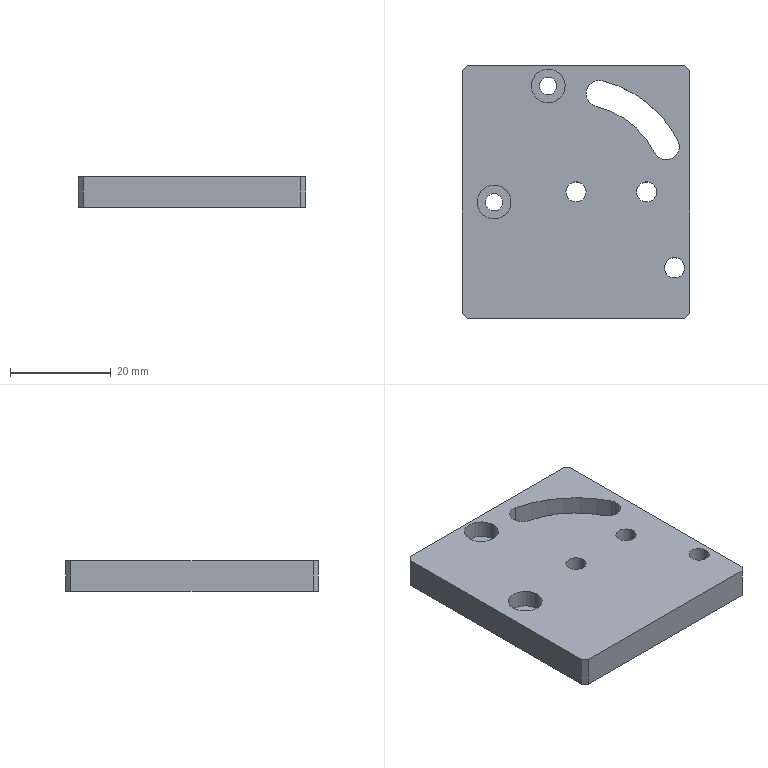Part | NX | features BREP 1 | 1 solid | 31 faces | box 45 x 50 x 6 mm | volume 12298 mm3 | cylinder 19 | plane 12 | commonest cylinder face diameters 4 x6 3.4 x4 6.7 x4 5.2 x3 34.8 x1 45.2 x1
STEP:
#1=CARTESIAN_POINT('',(-8.85,21.,2.5));
#2=VERTEX_POINT('',#1);
#3=CARTESIAN_POINT('',(-2.15,21.,2.5));
#4=VERTEX_POINT('',#3);
#5=CARTESIAN_POINT('',(-5.5,21.,2.5));
#6=DIRECTION('',(0.,0.,1.));
#7=DIRECTION('',(1.,0.,0.));
#8=AXIS2_PLACEMENT_3D('',#5,#6,#7);
#9=CIRCLE('',#8,3.35);
#10=EDGE_CURVE('',#2,#4,#9,.T.);
#11=ORIENTED_EDGE('',*,*,#10,.F.);
#12=CARTESIAN_POINT('',(-8.85,21.,6.));
#13=VERTEX_POINT('',#12);
#14=CARTESIAN_POINT('',(-8.85,21.,6.));
#15=DIRECTION('',(0.,0.,1.));
#16=VECTOR('',#15,1000.);
#17=LINE('',#14,#16);
#18=EDGE_CURVE('',#13,#2,#17,.F.);
#19=ORIENTED_EDGE('',*,*,#18,.F.);
#20=CARTESIAN_POINT('',(-2.15,21.,6.));
#21=VERTEX_POINT('',#20);
#22=CARTESIAN_POINT('',(-5.5,21.,6.));
#23=DIRECTION('',(0.,0.,1.));
#24=DIRECTION('',(1.,0.,0.));
#25=AXIS2_PLACEMENT_3D('',#22,#23,#24);
#26=CIRCLE('',#25,3.35);
#27=EDGE_CURVE('',#13,#21,#26,.T.);
#28=ORIENTED_EDGE('',*,*,#27,.T.);
#29=CARTESIAN_POINT('',(-2.15,21.,6.));
#30=DIRECTION('',(0.,0.,1.));
#31=VECTOR('',#30,1000.);
#32=LINE('',#29,#31);
#33=EDGE_CURVE('',#21,#4,#32,.F.);
#34=ORIENTED_EDGE('',*,*,#33,.T.);
#35=EDGE_LOOP('',(#11,#19,#28,#34));
#36=FACE_BOUND('',#35,.T.);
#37=CARTESIAN_POINT('',(-5.5,21.,6.));
#38=DIRECTION('',(0.,0.,1.));
#39=DIRECTION('',(1.,0.,0.));
#40=AXIS2_PLACEMENT_3D('',#37,#38,#39);
#41=CYLINDRICAL_SURFACE('',#40,3.35);
#42=ADVANCED_FACE('',(#36),#41,.F.);
#43=CARTESIAN_POINT('',(-7.2,21.,0.));
#44=VERTEX_POINT('',#43);
#45=CARTESIAN_POINT('',(-3.8,21.,0.));
#46=VERTEX_POINT('',#45);
#47=CARTESIAN_POINT('',(-5.5,21.,0.));
#48=DIRECTION('',(0.,0.,1.));
#49=DIRECTION('',(1.,0.,0.));
#50=AXIS2_PLACEMENT_3D('',#47,#48,#49);
#51=CIRCLE('',#50,1.7);
#52=EDGE_CURVE('',#44,#46,#51,.T.);
#53=ORIENTED_EDGE('',*,*,#52,.F.);
#54=CARTESIAN_POINT('',(-7.2,21.,2.5));
#55=VERTEX_POINT('',#54);
#56=CARTESIAN_POINT('',(-7.2,21.,6.));
#57=DIRECTION('',(0.,0.,1.));
#58=VECTOR('',#57,1000.);
#59=LINE('',#56,#58);
#60=EDGE_CURVE('',#55,#44,#59,.F.);
#61=ORIENTED_EDGE('',*,*,#60,.F.);
#62=CARTESIAN_POINT('',(-3.8,21.,2.5));
#63=VERTEX_POINT('',#62);
#64=CARTESIAN_POINT('',(-5.5,21.,2.5));
#65=DIRECTION('',(0.,0.,1.));
#66=DIRECTION('',(1.,0.,0.));
#67=AXIS2_PLACEMENT_3D('',#64,#65,#66);
#68=CIRCLE('',#67,1.7);
#69=EDGE_CURVE('',#55,#63,#68,.T.);
#70=ORIENTED_EDGE('',*,*,#69,.T.);
#71=CARTESIAN_POINT('',(-3.8,21.,6.));
#72=DIRECTION('',(0.,0.,1.));
#73=VECTOR('',#72,1000.);
#74=LINE('',#71,#73);
#75=EDGE_CURVE('',#63,#46,#74,.F.);
#76=ORIENTED_EDGE('',*,*,#75,.T.);
#77=EDGE_LOOP('',(#53,#61,#70,#76));
#78=FACE_BOUND('',#77,.T.);
#79=CARTESIAN_POINT('',(-5.5,21.,6.));
#80=DIRECTION('',(0.,0.,1.));
#81=DIRECTION('',(1.,0.,0.));
#82=AXIS2_PLACEMENT_3D('',#79,#80,#81);
#83=CYLINDRICAL_SURFACE('',#82,1.7);
#84=ADVANCED_FACE('',(#78),#83,.F.);
#85=CARTESIAN_POINT('',(-19.575,-2.,2.5));
#86=VERTEX_POINT('',#85);
#87=CARTESIAN_POINT('',(-12.875,-2.,2.5));
#88=VERTEX_POINT('',#87);
#89=CARTESIAN_POINT('',(-16.225,-2.,2.5));
#90=DIRECTION('',(0.,0.,1.));
#91=DIRECTION('',(1.,0.,0.));
#92=AXIS2_PLACEMENT_3D('',#89,#90,#91);
#93=CIRCLE('',#92,3.35);
#94=EDGE_CURVE('',#86,#88,#93,.T.);
#95=ORIENTED_EDGE('',*,*,#94,.F.);
#96=CARTESIAN_POINT('',(-19.575,-2.,6.));
#97=VERTEX_POINT('',#96);
#98=CARTESIAN_POINT('',(-19.575,-2.,6.));
#99=DIRECTION('',(0.,0.,1.));
#100=VECTOR('',#99,1000.);
#101=LINE('',#98,#100);
#102=EDGE_CURVE('',#97,#86,#101,.F.);
#103=ORIENTED_EDGE('',*,*,#102,.F.);
#104=CARTESIAN_POINT('',(-12.875,-2.,6.));
#105=VERTEX_POINT('',#104);
#106=CARTESIAN_POINT('',(-16.225,-2.,6.));
#107=DIRECTION('',(0.,0.,1.));
#108=DIRECTION('',(1.,0.,0.));
#109=AXIS2_PLACEMENT_3D('',#106,#107,#108);
#110=CIRCLE('',#109,3.35);
#111=EDGE_CURVE('',#97,#105,#110,.T.);
#112=ORIENTED_EDGE('',*,*,#111,.T.);
#113=CARTESIAN_POINT('',(-12.875,-2.,6.));
#114=DIRECTION('',(0.,0.,1.));
#115=VECTOR('',#114,1000.);
#116=LINE('',#113,#115);
#117=EDGE_CURVE('',#105,#88,#116,.F.);
#118=ORIENTED_EDGE('',*,*,#117,.T.);
#119=EDGE_LOOP('',(#95,#103,#112,#118));
#120=FACE_BOUND('',#119,.T.);
#121=CARTESIAN_POINT('',(-16.225,-2.,6.));
#122=DIRECTION('',(0.,0.,1.));
#123=DIRECTION('',(1.,0.,0.));
#124=AXIS2_PLACEMENT_3D('',#121,#122,#123);
#125=CYLINDRICAL_SURFACE('',#124,3.35);
#126=ADVANCED_FACE('',(#120),#125,.F.);
#127=CARTESIAN_POINT('',(-17.925,-2.,0.));
#128=VERTEX_POINT('',#127);
#129=CARTESIAN_POINT('',(-14.525,-2.,0.));
#130=VERTEX_POINT('',#129);
#131=CARTESIAN_POINT('',(-16.225,-2.,0.));
#132=DIRECTION('',(0.,0.,1.));
#133=DIRECTION('',(1.,0.,0.));
#134=AXIS2_PLACEMENT_3D('',#131,#132,#133);
#135=CIRCLE('',#134,1.7);
#136=EDGE_CURVE('',#128,#130,#135,.T.);
#137=ORIENTED_EDGE('',*,*,#136,.F.);
#138=CARTESIAN_POINT('',(-17.925,-2.,2.5));
#139=VERTEX_POINT('',#138);
#140=CARTESIAN_POINT('',(-17.925,-2.,6.));
#141=DIRECTION('',(0.,0.,1.));
#142=VECTOR('',#141,1000.);
#143=LINE('',#140,#142);
#144=EDGE_CURVE('',#139,#128,#143,.F.);
#145=ORIENTED_EDGE('',*,*,#144,.F.);
#146=CARTESIAN_POINT('',(-14.525,-2.,2.5));
#147=VERTEX_POINT('',#146);
#148=CARTESIAN_POINT('',(-16.225,-2.,2.5));
#149=DIRECTION('',(0.,0.,1.));
#150=DIRECTION('',(1.,0.,0.));
#151=AXIS2_PLACEMENT_3D('',#148,#149,#150);
#152=CIRCLE('',#151,1.7);
#153=EDGE_CURVE('',#139,#147,#152,.T.);
#154=ORIENTED_EDGE('',*,*,#153,.T.);
#155=CARTESIAN_POINT('',(-14.525,-2.,6.));
#156=DIRECTION('',(0.,0.,1.));
#157=VECTOR('',#156,1000.);
#158=LINE('',#155,#157);
#159=EDGE_CURVE('',#147,#130,#158,.F.);
#160=ORIENTED_EDGE('',*,*,#159,.T.);
#161=EDGE_LOOP('',(#137,#145,#154,#160));
#162=FACE_BOUND('',#161,.T.);
#163=CARTESIAN_POINT('',(-16.225,-2.,6.));
#164=DIRECTION('',(0.,0.,1.));
#165=DIRECTION('',(1.,0.,0.));
#166=AXIS2_PLACEMENT_3D('',#163,#164,#165);
#167=CYLINDRICAL_SURFACE('',#166,1.7);
#168=ADVANCED_FACE('',(#162),#167,.F.);
#169=CARTESIAN_POINT('',(17.5,-15.,6.));
#170=VERTEX_POINT('',#169);
#171=CARTESIAN_POINT('',(21.5,-15.,6.));
#172=VERTEX_POINT('',#171);
#173=CARTESIAN_POINT('',(19.5,-15.,6.));
#174=DIRECTION('',(0.,0.,1.));
#175=DIRECTION('',(1.,0.,0.));
#176=AXIS2_PLACEMENT_3D('',#173,#174,#175);
#177=CIRCLE('',#176,2.);
#178=EDGE_CURVE('',#170,#172,#177,.T.);
#179=ORIENTED_EDGE('',*,*,#178,.T.);
#180=CARTESIAN_POINT('',(21.5,-15.,0.));
#181=VERTEX_POINT('',#180);
#182=CARTESIAN_POINT('',(21.5,-15.,10.));
#183=DIRECTION('',(0.,0.,-1.));
#184=VECTOR('',#183,1000.);
#185=LINE('',#182,#184);
#186=EDGE_CURVE('',#172,#181,#185,.T.);
#187=ORIENTED_EDGE('',*,*,#186,.T.);
#188=CARTESIAN_POINT('',(17.5,-15.,0.));
#189=VERTEX_POINT('',#188);
#190=CARTESIAN_POINT('',(19.5,-15.,0.));
#191=DIRECTION('',(0.,0.,-1.));
#192=DIRECTION('',(-1.,0.,0.));
#193=AXIS2_PLACEMENT_3D('',#190,#191,#192);
#194=CIRCLE('',#193,2.);
#195=EDGE_CURVE('',#181,#189,#194,.T.);
#196=ORIENTED_EDGE('',*,*,#195,.T.);
#197=CARTESIAN_POINT('',(17.5,-15.,10.));
#198=DIRECTION('',(0.,0.,-1.));
#199=VECTOR('',#198,1000.);
#200=LINE('',#197,#199);
#201=EDGE_CURVE('',#170,#189,#200,.T.);
#202=ORIENTED_EDGE('',*,*,#201,.F.);
#203=EDGE_LOOP('',(#179,#187,#196,#202));
#204=FACE_BOUND('',#203,.T.);
#205=CARTESIAN_POINT('',(19.5,-15.,10.));
#206=DIRECTION('',(0.,0.,-1.));
#207=DIRECTION('',(-1.,0.,0.));
#208=AXIS2_PLACEMENT_3D('',#205,#206,#207);
#209=CYLINDRICAL_SURFACE('',#208,2.);
#210=ADVANCED_FACE('',(#204),#209,.F.);
#211=CARTESIAN_POINT('',(12.,0.,6.));
#212=VERTEX_POINT('',#211);
#213=CARTESIAN_POINT('',(16.,0.,6.));
#214=VERTEX_POINT('',#213);
#215=CARTESIAN_POINT('',(14.,0.,6.));
#216=DIRECTION('',(0.,0.,1.));
#217=DIRECTION('',(1.,0.,0.));
#218=AXIS2_PLACEMENT_3D('',#215,#216,#217);
#219=CIRCLE('',#218,2.);
#220=EDGE_CURVE('',#212,#214,#219,.T.);
#221=ORIENTED_EDGE('',*,*,#220,.T.);
#222=CARTESIAN_POINT('',(16.,0.,0.));
#223=VERTEX_POINT('',#222);
#224=CARTESIAN_POINT('',(16.,0.,10.));
#225=DIRECTION('',(0.,0.,-1.));
#226=VECTOR('',#225,1000.);
#227=LINE('',#224,#226);
#228=EDGE_CURVE('',#214,#223,#227,.T.);
#229=ORIENTED_EDGE('',*,*,#228,.T.);
#230=CARTESIAN_POINT('',(12.,0.,0.));
#231=VERTEX_POINT('',#230);
#232=CARTESIAN_POINT('',(14.,0.,0.));
#233=DIRECTION('',(0.,0.,-1.));
#234=DIRECTION('',(-1.,0.,0.));
#235=AXIS2_PLACEMENT_3D('',#232,#233,#234);
#236=CIRCLE('',#235,2.);
#237=EDGE_CURVE('',#223,#231,#236,.T.);
#238=ORIENTED_EDGE('',*,*,#237,.T.);
#239=CARTESIAN_POINT('',(12.,0.,10.));
#240=DIRECTION('',(0.,0.,-1.));
#241=VECTOR('',#240,1000.);
#242=LINE('',#239,#241);
#243=EDGE_CURVE('',#212,#231,#242,.T.);
#244=ORIENTED_EDGE('',*,*,#243,.F.);
#245=EDGE_LOOP('',(#221,#229,#238,#244));
#246=FACE_BOUND('',#245,.T.);
#247=CARTESIAN_POINT('',(14.,0.,10.));
#248=DIRECTION('',(0.,0.,-1.));
#249=DIRECTION('',(-1.,0.,0.));
#250=AXIS2_PLACEMENT_3D('',#247,#248,#249);
#251=CYLINDRICAL_SURFACE('',#250,2.);
#252=ADVANCED_FACE('',(#246),#251,.F.);
#253=CARTESIAN_POINT('',(5.182,21.998,6.));
#254=VERTEX_POINT('',#253);
#255=CARTESIAN_POINT('',(1.986,19.467,6.));
#256=VERTEX_POINT('',#255);
#257=CARTESIAN_POINT('',(4.586,19.467,6.));
#258=DIRECTION('',(0.,0.,1.));
#259=DIRECTION('',(1.,0.,0.));
#260=AXIS2_PLACEMENT_3D('',#257,#258,#259);
#261=CIRCLE('',#260,2.6);
#262=EDGE_CURVE('',#254,#256,#261,.T.);
#263=ORIENTED_EDGE('',*,*,#262,.T.);
#264=CARTESIAN_POINT('',(1.986,19.467,0.));
#265=VERTEX_POINT('',#264);
#266=CARTESIAN_POINT('',(1.986,19.467,10.));
#267=DIRECTION('',(0.,0.,-1.));
#268=VECTOR('',#267,1000.);
#269=LINE('',#266,#268);
#270=EDGE_CURVE('',#256,#265,#269,.T.);
#271=ORIENTED_EDGE('',*,*,#270,.T.);
#272=CARTESIAN_POINT('',(5.182,21.998,0.));
#273=VERTEX_POINT('',#272);
#274=CARTESIAN_POINT('',(4.586,19.467,0.));
#275=DIRECTION('',(0.,0.,-1.));
#276=DIRECTION('',(-1.,0.,0.));
#277=AXIS2_PLACEMENT_3D('',#274,#275,#276);
#278=CIRCLE('',#277,2.6);
#279=EDGE_CURVE('',#265,#273,#278,.T.);
#280=ORIENTED_EDGE('',*,*,#279,.T.);
#281=CARTESIAN_POINT('',(5.182,21.998,10.));
#282=DIRECTION('',(0.,0.,-1.));
#283=VECTOR('',#282,1000.);
#284=LINE('',#281,#283);
#285=EDGE_CURVE('',#254,#273,#284,.T.);
#286=ORIENTED_EDGE('',*,*,#285,.F.);
#287=EDGE_LOOP('',(#263,#271,#280,#286));
#288=FACE_BOUND('',#287,.T.);
#289=CARTESIAN_POINT('',(4.586,19.467,10.));
#290=DIRECTION('',(0.,0.,-1.));
#291=DIRECTION('',(-1.,0.,0.));
#292=AXIS2_PLACEMENT_3D('',#289,#290,#291);
#293=CYLINDRICAL_SURFACE('',#292,2.6);
#294=ADVANCED_FACE('',(#288),#293,.F.);
#295=CARTESIAN_POINT('',(-2.,0.,6.));
#296=VERTEX_POINT('',#295);
#297=CARTESIAN_POINT('',(2.,0.,6.));
#298=VERTEX_POINT('',#297);
#299=CARTESIAN_POINT('',(0.,0.,6.));
#300=DIRECTION('',(0.,0.,1.));
#301=DIRECTION('',(1.,0.,0.));
#302=AXIS2_PLACEMENT_3D('',#299,#300,#301);
#303=CIRCLE('',#302,2.);
#304=EDGE_CURVE('',#296,#298,#303,.T.);
#305=ORIENTED_EDGE('',*,*,#304,.T.);
#306=CARTESIAN_POINT('',(2.,0.,0.));
#307=VERTEX_POINT('',#306);
#308=CARTESIAN_POINT('',(2.,0.,10.));
#309=DIRECTION('',(0.,0.,-1.));
#310=VECTOR('',#309,1000.);
#311=LINE('',#308,#310);
#312=EDGE_CURVE('',#298,#307,#311,.T.);
#313=ORIENTED_EDGE('',*,*,#312,.T.);
#314=CARTESIAN_POINT('',(-2.,0.,0.));
#315=VERTEX_POINT('',#314);
#316=CARTESIAN_POINT('',(0.,0.,0.));
#317=DIRECTION('',(0.,0.,-1.));
#318=DIRECTION('',(-1.,0.,0.));
#319=AXIS2_PLACEMENT_3D('',#316,#317,#318);
#320=CIRCLE('',#319,2.);
#321=EDGE_CURVE('',#307,#315,#320,.T.);
#322=ORIENTED_EDGE('',*,*,#321,.T.);
#323=CARTESIAN_POINT('',(-2.,0.,10.));
#324=DIRECTION('',(0.,0.,-1.));
#325=VECTOR('',#324,1000.);
#326=LINE('',#323,#325);
#327=EDGE_CURVE('',#296,#315,#326,.T.);
#328=ORIENTED_EDGE('',*,*,#327,.F.);
#329=EDGE_LOOP('',(#305,#313,#322,#328));
#330=FACE_BOUND('',#329,.T.);
#331=CARTESIAN_POINT('',(0.,0.,10.));
#332=DIRECTION('',(0.,0.,-1.));
#333=DIRECTION('',(-1.,0.,0.));
#334=AXIS2_PLACEMENT_3D('',#331,#332,#333);
#335=CYLINDRICAL_SURFACE('',#334,2.);
#336=ADVANCED_FACE('',(#330),#335,.F.);
#337=CARTESIAN_POINT('',(22.5,-24.,6.));
#338=VERTEX_POINT('',#337);
#339=CARTESIAN_POINT('',(22.5,24.,6.));
#340=VERTEX_POINT('',#339);
#341=CARTESIAN_POINT('',(22.5,25.,6.));
#342=DIRECTION('',(0.,1.,0.));
#343=VECTOR('',#342,1000.);
#344=LINE('',#341,#343);
#345=EDGE_CURVE('',#338,#340,#344,.T.);
#346=ORIENTED_EDGE('',*,*,#345,.F.);
#347=CARTESIAN_POINT('',(22.5,-24.,0.));
#348=VERTEX_POINT('',#347);
#349=CARTESIAN_POINT('',(22.5,-24.,6.));
#350=DIRECTION('',(0.,0.,-1.));
#351=VECTOR('',#350,1000.);
#352=LINE('',#349,#351);
#353=EDGE_CURVE('',#338,#348,#352,.T.);
#354=ORIENTED_EDGE('',*,*,#353,.T.);
#355=CARTESIAN_POINT('',(22.5,24.,0.));
#356=VERTEX_POINT('',#355);
#357=CARTESIAN_POINT('',(22.5,25.,0.));
#358=DIRECTION('',(0.,1.,0.));
#359=VECTOR('',#358,1000.);
#360=LINE('',#357,#359);
#361=EDGE_CURVE('',#348,#356,#360,.T.);
#362=ORIENTED_EDGE('',*,*,#361,.T.);
#363=CARTESIAN_POINT('',(22.5,24.,6.));
#364=DIRECTION('',(0.,0.,1.));
#365=VECTOR('',#364,1000.);
#366=LINE('',#363,#365);
#367=EDGE_CURVE('',#356,#340,#366,.T.);
#368=ORIENTED_EDGE('',*,*,#367,.T.);
#369=EDGE_LOOP('',(#346,#354,#362,#368));
#370=FACE_BOUND('',#369,.T.);
#371=CARTESIAN_POINT('',(22.5,25.,6.));
#372=DIRECTION('',(-1.,0.,0.));
#373=DIRECTION('',(0.,1.,0.));
#374=AXIS2_PLACEMENT_3D('',#371,#372,#373);
#375=PLANE('',#374);
#376=ADVANCED_FACE('',(#370),#375,.F.);
#377=CARTESIAN_POINT('',(21.5,25.,0.));
#378=VERTEX_POINT('',#377);
#379=CARTESIAN_POINT('',(-21.5,25.,0.));
#380=VERTEX_POINT('',#379);
#381=CARTESIAN_POINT('',(-22.5,25.,0.));
#382=DIRECTION('',(-1.,0.,0.));
#383=VECTOR('',#382,1000.);
#384=LINE('',#381,#383);
#385=EDGE_CURVE('',#378,#380,#384,.T.);
#386=ORIENTED_EDGE('',*,*,#385,.T.);
#387=CARTESIAN_POINT('',(-21.5,25.,6.));
#388=VERTEX_POINT('',#387);
#389=CARTESIAN_POINT('',(-21.5,25.,6.));
#390=DIRECTION('',(0.,0.,1.));
#391=VECTOR('',#390,1000.);
#392=LINE('',#389,#391);
#393=EDGE_CURVE('',#380,#388,#392,.T.);
#394=ORIENTED_EDGE('',*,*,#393,.T.);
#395=CARTESIAN_POINT('',(21.5,25.,6.));
#396=VERTEX_POINT('',#395);
#397=CARTESIAN_POINT('',(-22.5,25.,6.));
#398=DIRECTION('',(-1.,0.,0.));
#399=VECTOR('',#398,1000.);
#400=LINE('',#397,#399);
#401=EDGE_CURVE('',#396,#388,#400,.T.);
#402=ORIENTED_EDGE('',*,*,#401,.F.);
#403=CARTESIAN_POINT('',(21.5,25.,6.));
#404=DIRECTION('',(0.,0.,-1.));
#405=VECTOR('',#404,1000.);
#406=LINE('',#403,#405);
#407=EDGE_CURVE('',#396,#378,#406,.T.);
#408=ORIENTED_EDGE('',*,*,#407,.T.);
#409=EDGE_LOOP('',(#386,#394,#402,#408));
#410=FACE_BOUND('',#409,.T.);
#411=CARTESIAN_POINT('',(-22.5,25.,6.));
#412=DIRECTION('',(0.,-1.,0.));
#413=DIRECTION('',(0.,0.,-1.));
#414=AXIS2_PLACEMENT_3D('',#411,#412,#413);
#415=PLANE('',#414);
#416=ADVANCED_FACE('',(#410),#415,.F.);
#417=CARTESIAN_POINT('',(-22.5,24.,0.));
#418=VERTEX_POINT('',#417);
#419=CARTESIAN_POINT('',(-22.5,-24.,0.));
#420=VERTEX_POINT('',#419);
#421=CARTESIAN_POINT('',(-22.5,25.,0.));
#422=DIRECTION('',(0.,-1.,0.));
#423=VECTOR('',#422,1000.);
#424=LINE('',#421,#423);
#425=EDGE_CURVE('',#418,#420,#424,.T.);
#426=ORIENTED_EDGE('',*,*,#425,.T.);
#427=CARTESIAN_POINT('',(-22.5,-24.,6.));
#428=VERTEX_POINT('',#427);
#429=CARTESIAN_POINT('',(-22.5,-24.,6.));
#430=DIRECTION('',(0.,0.,1.));
#431=VECTOR('',#430,1000.);
#432=LINE('',#429,#431);
#433=EDGE_CURVE('',#420,#428,#432,.T.);
#434=ORIENTED_EDGE('',*,*,#433,.T.);
#435=CARTESIAN_POINT('',(-22.5,24.,6.));
#436=VERTEX_POINT('',#435);
#437=CARTESIAN_POINT('',(-22.5,25.,6.));
#438=DIRECTION('',(0.,-1.,0.));
#439=VECTOR('',#438,1000.);
#440=LINE('',#437,#439);
#441=EDGE_CURVE('',#436,#428,#440,.T.);
#442=ORIENTED_EDGE('',*,*,#441,.F.);
#443=CARTESIAN_POINT('',(-22.5,24.,6.));
#444=DIRECTION('',(0.,0.,-1.));
#445=VECTOR('',#444,1000.);
#446=LINE('',#443,#445);
#447=EDGE_CURVE('',#436,#418,#446,.T.);
#448=ORIENTED_EDGE('',*,*,#447,.T.);
#449=EDGE_LOOP('',(#426,#434,#442,#448));
#450=FACE_BOUND('',#449,.T.);
#451=CARTESIAN_POINT('',(-22.5,25.,6.));
#452=DIRECTION('',(1.,0.,0.));
#453=DIRECTION('',(0.,1.,0.));
#454=AXIS2_PLACEMENT_3D('',#451,#452,#453);
#455=PLANE('',#454);
#456=ADVANCED_FACE('',(#450),#455,.F.);
#457=CARTESIAN_POINT('',(-21.5,-25.,6.));
#458=VERTEX_POINT('',#457);
#459=CARTESIAN_POINT('',(21.5,-25.,6.));
#460=VERTEX_POINT('',#459);
#461=CARTESIAN_POINT('',(-22.5,-25.,6.));
#462=DIRECTION('',(1.,0.,0.));
#463=VECTOR('',#462,1000.);
#464=LINE('',#461,#463);
#465=EDGE_CURVE('',#458,#460,#464,.T.);
#466=ORIENTED_EDGE('',*,*,#465,.F.);
#467=CARTESIAN_POINT('',(-21.5,-25.,0.));
#468=VERTEX_POINT('',#467);
#469=CARTESIAN_POINT('',(-21.5,-25.,6.));
#470=DIRECTION('',(0.,0.,-1.));
#471=VECTOR('',#470,1000.);
#472=LINE('',#469,#471);
#473=EDGE_CURVE('',#458,#468,#472,.T.);
#474=ORIENTED_EDGE('',*,*,#473,.T.);
#475=CARTESIAN_POINT('',(21.5,-25.,0.));
#476=VERTEX_POINT('',#475);
#477=CARTESIAN_POINT('',(-22.5,-25.,0.));
#478=DIRECTION('',(1.,0.,0.));
#479=VECTOR('',#478,1000.);
#480=LINE('',#477,#479);
#481=EDGE_CURVE('',#468,#476,#480,.T.);
#482=ORIENTED_EDGE('',*,*,#481,.T.);
#483=CARTESIAN_POINT('',(21.5,-25.,6.));
#484=DIRECTION('',(0.,0.,1.));
#485=VECTOR('',#484,1000.);
#486=LINE('',#483,#485);
#487=EDGE_CURVE('',#476,#460,#486,.T.);
#488=ORIENTED_EDGE('',*,*,#487,.T.);
#489=EDGE_LOOP('',(#466,#474,#482,#488));
#490=FACE_BOUND('',#489,.T.);
#491=CARTESIAN_POINT('',(-22.5,-25.,6.));
#492=DIRECTION('',(0.,1.,0.));
#493=DIRECTION('',(1.,0.,0.));
#494=AXIS2_PLACEMENT_3D('',#491,#492,#493);
#495=PLANE('',#494);
#496=ADVANCED_FACE('',(#490),#495,.F.);
#497=ORIENTED_EDGE('',*,*,#441,.T.);
#498=CARTESIAN_POINT('',(-23.25,-23.25,6.));
#499=DIRECTION('',(0.7071,-0.7071,0.));
#500=VECTOR('',#499,1000.);
#501=LINE('',#498,#500);
#502=EDGE_CURVE('',#428,#458,#501,.T.);
#503=ORIENTED_EDGE('',*,*,#502,.T.);
#504=ORIENTED_EDGE('',*,*,#465,.T.);
#505=CARTESIAN_POINT('',(23.25,-23.25,6.));
#506=DIRECTION('',(0.7071,0.7071,0.));
#507=VECTOR('',#506,1000.);
#508=LINE('',#505,#507);
#509=EDGE_CURVE('',#460,#338,#508,.T.);
#510=ORIENTED_EDGE('',*,*,#509,.T.);
#511=ORIENTED_EDGE('',*,*,#345,.T.);
#512=CARTESIAN_POINT('',(23.25,23.25,6.));
#513=DIRECTION('',(-0.7071,0.7071,0.));
#514=VECTOR('',#513,1000.);
#515=LINE('',#512,#514);
#516=EDGE_CURVE('',#340,#396,#515,.T.);
#517=ORIENTED_EDGE('',*,*,#516,.T.);
#518=ORIENTED_EDGE('',*,*,#401,.T.);
#519=CARTESIAN_POINT('',(-23.25,23.25,6.));
#520=DIRECTION('',(-0.7071,-0.7071,0.));
#521=VECTOR('',#520,1000.);
#522=LINE('',#519,#521);
#523=EDGE_CURVE('',#388,#436,#522,.T.);
#524=ORIENTED_EDGE('',*,*,#523,.T.);
#525=EDGE_LOOP('',(#497,#503,#504,#510,#511,#517,#518,#524));
#526=FACE_BOUND('',#525,.T.);
#527=CARTESIAN_POINT('',(-5.5,21.,6.));
#528=DIRECTION('',(0.,0.,1.));
#529=DIRECTION('',(1.,0.,0.));
#530=AXIS2_PLACEMENT_3D('',#527,#528,#529);
#531=CIRCLE('',#530,3.35);
#532=EDGE_CURVE('',#21,#13,#531,.T.);
#533=ORIENTED_EDGE('',*,*,#532,.F.);
#534=ORIENTED_EDGE('',*,*,#27,.F.);
#535=EDGE_LOOP('',(#533,#534));
#536=FACE_BOUND('',#535,.T.);
#537=CARTESIAN_POINT('',(-16.225,-2.,6.));
#538=DIRECTION('',(0.,0.,1.));
#539=DIRECTION('',(1.,0.,0.));
#540=AXIS2_PLACEMENT_3D('',#537,#538,#539);
#541=CIRCLE('',#540,3.35);
#542=EDGE_CURVE('',#105,#97,#541,.T.);
#543=ORIENTED_EDGE('',*,*,#542,.F.);
#544=ORIENTED_EDGE('',*,*,#111,.F.);
#545=EDGE_LOOP('',(#543,#544));
#546=FACE_BOUND('',#545,.T.);
#547=ORIENTED_EDGE('',*,*,#178,.F.);
#548=CARTESIAN_POINT('',(19.5,-15.,6.));
#549=DIRECTION('',(0.,0.,1.));
#550=DIRECTION('',(1.,0.,0.));
#551=AXIS2_PLACEMENT_3D('',#548,#549,#550);
#552=CIRCLE('',#551,2.);
#553=EDGE_CURVE('',#172,#170,#552,.T.);
#554=ORIENTED_EDGE('',*,*,#553,.F.);
#555=EDGE_LOOP('',(#547,#554));
#556=FACE_BOUND('',#555,.T.);
#557=ORIENTED_EDGE('',*,*,#220,.F.);
#558=CARTESIAN_POINT('',(14.,0.,6.));
#559=DIRECTION('',(0.,0.,1.));
#560=DIRECTION('',(1.,0.,0.));
#561=AXIS2_PLACEMENT_3D('',#558,#559,#560);
#562=CIRCLE('',#561,2.);
#563=EDGE_CURVE('',#214,#212,#562,.T.);
#564=ORIENTED_EDGE('',*,*,#563,.F.);
#565=EDGE_LOOP('',(#557,#564));
#566=FACE_BOUND('',#565,.T.);
#567=ORIENTED_EDGE('',*,*,#262,.F.);
#568=CARTESIAN_POINT('',(20.182,10.17,6.));
#569=VERTEX_POINT('',#568);
#570=CARTESIAN_POINT('',(0.,0.,6.));
#571=DIRECTION('',(0.,0.,1.));
#572=DIRECTION('',(1.,0.,0.));
#573=AXIS2_PLACEMENT_3D('',#570,#571,#572);
#574=CIRCLE('',#573,22.6);
#575=EDGE_CURVE('',#569,#254,#574,.T.);
#576=ORIENTED_EDGE('',*,*,#575,.F.);
#577=CARTESIAN_POINT('',(15.539,7.83,6.));
#578=VERTEX_POINT('',#577);
#579=CARTESIAN_POINT('',(17.861,9.,6.));
#580=DIRECTION('',(0.,0.,1.));
#581=DIRECTION('',(1.,0.,0.));
#582=AXIS2_PLACEMENT_3D('',#579,#580,#581);
#583=CIRCLE('',#582,2.6);
#584=EDGE_CURVE('',#578,#569,#583,.T.);
#585=ORIENTED_EDGE('',*,*,#584,.F.);
#586=CARTESIAN_POINT('',(3.99,16.936,6.));
#587=VERTEX_POINT('',#586);
#588=CARTESIAN_POINT('',(0.,0.,6.));
#589=DIRECTION('',(0.,0.,-1.));
#590=DIRECTION('',(1.,0.,0.));
#591=AXIS2_PLACEMENT_3D('',#588,#589,#590);
#592=CIRCLE('',#591,17.4);
#593=EDGE_CURVE('',#587,#578,#592,.T.);
#594=ORIENTED_EDGE('',*,*,#593,.F.);
#595=CARTESIAN_POINT('',(4.586,19.467,6.));
#596=DIRECTION('',(0.,0.,1.));
#597=DIRECTION('',(1.,0.,0.));
#598=AXIS2_PLACEMENT_3D('',#595,#596,#597);
#599=CIRCLE('',#598,2.6);
#600=EDGE_CURVE('',#256,#587,#599,.T.);
#601=ORIENTED_EDGE('',*,*,#600,.F.);
#602=EDGE_LOOP('',(#567,#576,#585,#594,#601));
#603=FACE_BOUND('',#602,.T.);
#604=ORIENTED_EDGE('',*,*,#304,.F.);
#605=CARTESIAN_POINT('',(0.,0.,6.));
#606=DIRECTION('',(0.,0.,1.));
#607=DIRECTION('',(1.,0.,0.));
#608=AXIS2_PLACEMENT_3D('',#605,#606,#607);
#609=CIRCLE('',#608,2.);
#610=EDGE_CURVE('',#298,#296,#609,.T.);
#611=ORIENTED_EDGE('',*,*,#610,.F.);
#612=EDGE_LOOP('',(#604,#611));
#613=FACE_BOUND('',#612,.T.);
#614=CARTESIAN_POINT('',(0.,0.,6.));
#615=DIRECTION('',(0.,0.,1.));
#616=DIRECTION('',(1.,0.,0.));
#617=AXIS2_PLACEMENT_3D('',#614,#615,#616);
#618=PLANE('',#617);
#619=ADVANCED_FACE('',(#526,#536,#546,#556,#566,#603,#613),#618,.T.);
#620=ORIENTED_EDGE('',*,*,#481,.F.);
#621=CARTESIAN_POINT('',(-21.5,-25.,0.));
#622=DIRECTION('',(-0.7071,0.7071,0.));
#623=VECTOR('',#622,1000.);
#624=LINE('',#621,#623);
#625=EDGE_CURVE('',#468,#420,#624,.T.);
#626=ORIENTED_EDGE('',*,*,#625,.T.);
#627=ORIENTED_EDGE('',*,*,#425,.F.);
#628=CARTESIAN_POINT('',(-22.5,24.,0.));
#629=DIRECTION('',(0.7071,0.7071,0.));
#630=VECTOR('',#629,1000.);
#631=LINE('',#628,#630);
#632=EDGE_CURVE('',#418,#380,#631,.T.);
#633=ORIENTED_EDGE('',*,*,#632,.T.);
#634=ORIENTED_EDGE('',*,*,#385,.F.);
#635=CARTESIAN_POINT('',(21.5,25.,0.));
#636=DIRECTION('',(0.7071,-0.7071,0.));
#637=VECTOR('',#636,1000.);
#638=LINE('',#635,#637);
#639=EDGE_CURVE('',#378,#356,#638,.T.);
#640=ORIENTED_EDGE('',*,*,#639,.T.);
#641=ORIENTED_EDGE('',*,*,#361,.F.);
#642=CARTESIAN_POINT('',(22.5,-24.,0.));
#643=DIRECTION('',(-0.7071,-0.7071,0.));
#644=VECTOR('',#643,1000.);
#645=LINE('',#642,#644);
#646=EDGE_CURVE('',#348,#476,#645,.T.);
#647=ORIENTED_EDGE('',*,*,#646,.T.);
#648=EDGE_LOOP('',(#620,#626,#627,#633,#634,#640,#641,#647));
#649=FACE_BOUND('',#648,.T.);
#650=CARTESIAN_POINT('',(-5.5,21.,0.));
#651=DIRECTION('',(0.,0.,1.));
#652=DIRECTION('',(1.,0.,0.));
#653=AXIS2_PLACEMENT_3D('',#650,#651,#652);
#654=CIRCLE('',#653,1.7);
#655=EDGE_CURVE('',#46,#44,#654,.T.);
#656=ORIENTED_EDGE('',*,*,#655,.T.);
#657=ORIENTED_EDGE('',*,*,#52,.T.);
#658=EDGE_LOOP('',(#656,#657));
#659=FACE_BOUND('',#658,.T.);
#660=CARTESIAN_POINT('',(-16.225,-2.,0.));
#661=DIRECTION('',(0.,0.,1.));
#662=DIRECTION('',(1.,0.,0.));
#663=AXIS2_PLACEMENT_3D('',#660,#661,#662);
#664=CIRCLE('',#663,1.7);
#665=EDGE_CURVE('',#130,#128,#664,.T.);
#666=ORIENTED_EDGE('',*,*,#665,.T.);
#667=ORIENTED_EDGE('',*,*,#136,.T.);
#668=EDGE_LOOP('',(#666,#667));
#669=FACE_BOUND('',#668,.T.);
#670=CARTESIAN_POINT('',(19.5,-15.,0.));
#671=DIRECTION('',(0.,0.,-1.));
#672=DIRECTION('',(-1.,0.,0.));
#673=AXIS2_PLACEMENT_3D('',#670,#671,#672);
#674=CIRCLE('',#673,2.);
#675=EDGE_CURVE('',#189,#181,#674,.T.);
#676=ORIENTED_EDGE('',*,*,#675,.F.);
#677=ORIENTED_EDGE('',*,*,#195,.F.);
#678=EDGE_LOOP('',(#676,#677));
#679=FACE_BOUND('',#678,.T.);
#680=CARTESIAN_POINT('',(14.,0.,0.));
#681=DIRECTION('',(0.,0.,-1.));
#682=DIRECTION('',(-1.,0.,0.));
#683=AXIS2_PLACEMENT_3D('',#680,#681,#682);
#684=CIRCLE('',#683,2.);
#685=EDGE_CURVE('',#231,#223,#684,.T.);
#686=ORIENTED_EDGE('',*,*,#685,.F.);
#687=ORIENTED_EDGE('',*,*,#237,.F.);
#688=EDGE_LOOP('',(#686,#687));
#689=FACE_BOUND('',#688,.T.);
#690=CARTESIAN_POINT('',(20.182,10.17,0.));
#691=VERTEX_POINT('',#690);
#692=CARTESIAN_POINT('',(0.,0.,0.));
#693=DIRECTION('',(0.,0.,-1.));
#694=DIRECTION('',(-1.,0.,0.));
#695=AXIS2_PLACEMENT_3D('',#692,#693,#694);
#696=CIRCLE('',#695,22.6);
#697=EDGE_CURVE('',#273,#691,#696,.T.);
#698=ORIENTED_EDGE('',*,*,#697,.F.);
#699=ORIENTED_EDGE('',*,*,#279,.F.);
#700=CARTESIAN_POINT('',(3.99,16.936,0.));
#701=VERTEX_POINT('',#700);
#702=CARTESIAN_POINT('',(4.586,19.467,0.));
#703=DIRECTION('',(0.,0.,-1.));
#704=DIRECTION('',(-1.,0.,0.));
#705=AXIS2_PLACEMENT_3D('',#702,#703,#704);
#706=CIRCLE('',#705,2.6);
#707=EDGE_CURVE('',#701,#265,#706,.T.);
#708=ORIENTED_EDGE('',*,*,#707,.F.);
#709=CARTESIAN_POINT('',(15.539,7.83,0.));
#710=VERTEX_POINT('',#709);
#711=CARTESIAN_POINT('',(0.,0.,0.));
#712=DIRECTION('',(0.,0.,1.));
#713=DIRECTION('',(-1.,0.,0.));
#714=AXIS2_PLACEMENT_3D('',#711,#712,#713);
#715=CIRCLE('',#714,17.4);
#716=EDGE_CURVE('',#710,#701,#715,.T.);
#717=ORIENTED_EDGE('',*,*,#716,.F.);
#718=CARTESIAN_POINT('',(17.861,9.,0.));
#719=DIRECTION('',(0.,0.,-1.));
#720=DIRECTION('',(-1.,0.,0.));
#721=AXIS2_PLACEMENT_3D('',#718,#719,#720);
#722=CIRCLE('',#721,2.6);
#723=EDGE_CURVE('',#691,#710,#722,.T.);
#724=ORIENTED_EDGE('',*,*,#723,.F.);
#725=EDGE_LOOP('',(#698,#699,#708,#717,#724));
#726=FACE_BOUND('',#725,.T.);
#727=CARTESIAN_POINT('',(0.,0.,0.));
#728=DIRECTION('',(0.,0.,-1.));
#729=DIRECTION('',(-1.,0.,0.));
#730=AXIS2_PLACEMENT_3D('',#727,#728,#729);
#731=CIRCLE('',#730,2.);
#732=EDGE_CURVE('',#315,#307,#731,.T.);
#733=ORIENTED_EDGE('',*,*,#732,.F.);
#734=ORIENTED_EDGE('',*,*,#321,.F.);
#735=EDGE_LOOP('',(#733,#734));
#736=FACE_BOUND('',#735,.T.);
#737=CARTESIAN_POINT('',(0.,0.,0.));
#738=DIRECTION('',(0.,0.,1.));
#739=DIRECTION('',(1.,0.,0.));
#740=AXIS2_PLACEMENT_3D('',#737,#738,#739);
#741=PLANE('',#740);
#742=ADVANCED_FACE('',(#649,#659,#669,#679,#689,#726,#736),#741,.F.);
#743=ORIENTED_EDGE('',*,*,#502,.F.);
#744=ORIENTED_EDGE('',*,*,#433,.F.);
#745=ORIENTED_EDGE('',*,*,#625,.F.);
#746=ORIENTED_EDGE('',*,*,#473,.F.);
#747=EDGE_LOOP('',(#743,#744,#745,#746));
#748=FACE_BOUND('',#747,.T.);
#749=CARTESIAN_POINT('',(-21.5,-25.,6.));
#750=DIRECTION('',(0.7071,0.7071,0.));
#751=DIRECTION('',(0.,0.,-1.));
#752=AXIS2_PLACEMENT_3D('',#749,#750,#751);
#753=PLANE('',#752);
#754=ADVANCED_FACE('',(#748),#753,.F.);
#755=ORIENTED_EDGE('',*,*,#509,.F.);
#756=ORIENTED_EDGE('',*,*,#487,.F.);
#757=ORIENTED_EDGE('',*,*,#646,.F.);
#758=ORIENTED_EDGE('',*,*,#353,.F.);
#759=EDGE_LOOP('',(#755,#756,#757,#758));
#760=FACE_BOUND('',#759,.T.);
#761=CARTESIAN_POINT('',(22.5,-24.,6.));
#762=DIRECTION('',(-0.7071,0.7071,0.));
#763=DIRECTION('',(0.,0.,1.));
#764=AXIS2_PLACEMENT_3D('',#761,#762,#763);
#765=PLANE('',#764);
#766=ADVANCED_FACE('',(#760),#765,.F.);
#767=ORIENTED_EDGE('',*,*,#523,.F.);
#768=ORIENTED_EDGE('',*,*,#393,.F.);
#769=ORIENTED_EDGE('',*,*,#632,.F.);
#770=ORIENTED_EDGE('',*,*,#447,.F.);
#771=EDGE_LOOP('',(#767,#768,#769,#770));
#772=FACE_BOUND('',#771,.T.);
#773=CARTESIAN_POINT('',(-22.5,24.,6.));
#774=DIRECTION('',(0.7071,-0.7071,0.));
#775=DIRECTION('',(0.,0.,-1.));
#776=AXIS2_PLACEMENT_3D('',#773,#774,#775);
#777=PLANE('',#776);
#778=ADVANCED_FACE('',(#772),#777,.F.);
#779=ORIENTED_EDGE('',*,*,#516,.F.);
#780=ORIENTED_EDGE('',*,*,#367,.F.);
#781=ORIENTED_EDGE('',*,*,#639,.F.);
#782=ORIENTED_EDGE('',*,*,#407,.F.);
#783=EDGE_LOOP('',(#779,#780,#781,#782));
#784=FACE_BOUND('',#783,.T.);
#785=CARTESIAN_POINT('',(21.5,25.,6.));
#786=DIRECTION('',(-0.7071,-0.7071,0.));
#787=DIRECTION('',(-0.7071,0.7071,0.));
#788=AXIS2_PLACEMENT_3D('',#785,#786,#787);
#789=PLANE('',#788);
#790=ADVANCED_FACE('',(#784),#789,.F.);
#791=ORIENTED_EDGE('',*,*,#312,.F.);
#792=ORIENTED_EDGE('',*,*,#610,.T.);
#793=ORIENTED_EDGE('',*,*,#327,.T.);
#794=ORIENTED_EDGE('',*,*,#732,.T.);
#795=EDGE_LOOP('',(#791,#792,#793,#794));
#796=FACE_BOUND('',#795,.T.);
#797=CARTESIAN_POINT('',(0.,0.,10.));
#798=DIRECTION('',(0.,0.,-1.));
#799=DIRECTION('',(-1.,0.,0.));
#800=AXIS2_PLACEMENT_3D('',#797,#798,#799);
#801=CYLINDRICAL_SURFACE('',#800,2.);
#802=ADVANCED_FACE('',(#796),#801,.F.);
#803=ORIENTED_EDGE('',*,*,#270,.F.);
#804=ORIENTED_EDGE('',*,*,#600,.T.);
#805=CARTESIAN_POINT('',(3.99,16.936,10.));
#806=DIRECTION('',(0.,0.,-1.));
#807=VECTOR('',#806,1000.);
#808=LINE('',#805,#807);
#809=EDGE_CURVE('',#587,#701,#808,.T.);
#810=ORIENTED_EDGE('',*,*,#809,.T.);
#811=ORIENTED_EDGE('',*,*,#707,.T.);
#812=EDGE_LOOP('',(#803,#804,#810,#811));
#813=FACE_BOUND('',#812,.T.);
#814=CARTESIAN_POINT('',(4.586,19.467,10.));
#815=DIRECTION('',(0.,0.,-1.));
#816=DIRECTION('',(-1.,0.,0.));
#817=AXIS2_PLACEMENT_3D('',#814,#815,#816);
#818=CYLINDRICAL_SURFACE('',#817,2.6);
#819=ADVANCED_FACE('',(#813),#818,.F.);
#820=ORIENTED_EDGE('',*,*,#593,.T.);
#821=CARTESIAN_POINT('',(15.539,7.83,10.));
#822=DIRECTION('',(0.,0.,-1.));
#823=VECTOR('',#822,1000.);
#824=LINE('',#821,#823);
#825=EDGE_CURVE('',#578,#710,#824,.T.);
#826=ORIENTED_EDGE('',*,*,#825,.T.);
#827=ORIENTED_EDGE('',*,*,#716,.T.);
#828=ORIENTED_EDGE('',*,*,#809,.F.);
#829=EDGE_LOOP('',(#820,#826,#827,#828));
#830=FACE_BOUND('',#829,.T.);
#831=CARTESIAN_POINT('',(0.,0.,10.));
#832=DIRECTION('',(0.,0.,-1.));
#833=DIRECTION('',(-1.,0.,0.));
#834=AXIS2_PLACEMENT_3D('',#831,#832,#833);
#835=CYLINDRICAL_SURFACE('',#834,17.4);
#836=ADVANCED_FACE('',(#830),#835,.T.);
#837=ORIENTED_EDGE('',*,*,#584,.T.);
#838=CARTESIAN_POINT('',(20.182,10.17,10.));
#839=DIRECTION('',(0.,0.,-1.));
#840=VECTOR('',#839,1000.);
#841=LINE('',#838,#840);
#842=EDGE_CURVE('',#569,#691,#841,.T.);
#843=ORIENTED_EDGE('',*,*,#842,.T.);
#844=ORIENTED_EDGE('',*,*,#723,.T.);
#845=ORIENTED_EDGE('',*,*,#825,.F.);
#846=EDGE_LOOP('',(#837,#843,#844,#845));
#847=FACE_BOUND('',#846,.T.);
#848=CARTESIAN_POINT('',(17.861,9.,10.));
#849=DIRECTION('',(0.,0.,-1.));
#850=DIRECTION('',(-1.,0.,0.));
#851=AXIS2_PLACEMENT_3D('',#848,#849,#850);
#852=CYLINDRICAL_SURFACE('',#851,2.6);
#853=ADVANCED_FACE('',(#847),#852,.F.);
#854=ORIENTED_EDGE('',*,*,#575,.T.);
#855=ORIENTED_EDGE('',*,*,#285,.T.);
#856=ORIENTED_EDGE('',*,*,#697,.T.);
#857=ORIENTED_EDGE('',*,*,#842,.F.);
#858=EDGE_LOOP('',(#854,#855,#856,#857));
#859=FACE_BOUND('',#858,.T.);
#860=CARTESIAN_POINT('',(0.,0.,10.));
#861=DIRECTION('',(0.,0.,-1.));
#862=DIRECTION('',(-1.,0.,0.));
#863=AXIS2_PLACEMENT_3D('',#860,#861,#862);
#864=CYLINDRICAL_SURFACE('',#863,22.6);
#865=ADVANCED_FACE('',(#859),#864,.F.);
#866=ORIENTED_EDGE('',*,*,#228,.F.);
#867=ORIENTED_EDGE('',*,*,#563,.T.);
#868=ORIENTED_EDGE('',*,*,#243,.T.);
#869=ORIENTED_EDGE('',*,*,#685,.T.);
#870=EDGE_LOOP('',(#866,#867,#868,#869));
#871=FACE_BOUND('',#870,.T.);
#872=CARTESIAN_POINT('',(14.,0.,10.));
#873=DIRECTION('',(0.,0.,-1.));
#874=DIRECTION('',(-1.,0.,0.));
#875=AXIS2_PLACEMENT_3D('',#872,#873,#874);
#876=CYLINDRICAL_SURFACE('',#875,2.);
#877=ADVANCED_FACE('',(#871),#876,.F.);
#878=ORIENTED_EDGE('',*,*,#186,.F.);
#879=ORIENTED_EDGE('',*,*,#553,.T.);
#880=ORIENTED_EDGE('',*,*,#201,.T.);
#881=ORIENTED_EDGE('',*,*,#675,.T.);
#882=EDGE_LOOP('',(#878,#879,#880,#881));
#883=FACE_BOUND('',#882,.T.);
#884=CARTESIAN_POINT('',(19.5,-15.,10.));
#885=DIRECTION('',(0.,0.,-1.));
#886=DIRECTION('',(-1.,0.,0.));
#887=AXIS2_PLACEMENT_3D('',#884,#885,#886);
#888=CYLINDRICAL_SURFACE('',#887,2.);
#889=ADVANCED_FACE('',(#883),#888,.F.);
#890=ORIENTED_EDGE('',*,*,#144,.T.);
#891=ORIENTED_EDGE('',*,*,#665,.F.);
#892=ORIENTED_EDGE('',*,*,#159,.F.);
#893=CARTESIAN_POINT('',(-16.225,-2.,2.5));
#894=DIRECTION('',(0.,0.,1.));
#895=DIRECTION('',(1.,0.,0.));
#896=AXIS2_PLACEMENT_3D('',#893,#894,#895);
#897=CIRCLE('',#896,1.7);
#898=EDGE_CURVE('',#147,#139,#897,.T.);
#899=ORIENTED_EDGE('',*,*,#898,.T.);
#900=EDGE_LOOP('',(#890,#891,#892,#899));
#901=FACE_BOUND('',#900,.T.);
#902=CARTESIAN_POINT('',(-16.225,-2.,6.));
#903=DIRECTION('',(0.,0.,1.));
#904=DIRECTION('',(1.,0.,0.));
#905=AXIS2_PLACEMENT_3D('',#902,#903,#904);
#906=CYLINDRICAL_SURFACE('',#905,1.7);
#907=ADVANCED_FACE('',(#901),#906,.F.);
#908=CARTESIAN_POINT('',(-16.225,-2.,2.5));
#909=DIRECTION('',(0.,0.,1.));
#910=DIRECTION('',(1.,0.,0.));
#911=AXIS2_PLACEMENT_3D('',#908,#909,#910);
#912=CIRCLE('',#911,3.35);
#913=EDGE_CURVE('',#88,#86,#912,.T.);
#914=ORIENTED_EDGE('',*,*,#913,.T.);
#915=ORIENTED_EDGE('',*,*,#94,.T.);
#916=EDGE_LOOP('',(#914,#915));
#917=FACE_BOUND('',#916,.T.);
#918=ORIENTED_EDGE('',*,*,#898,.F.);
#919=ORIENTED_EDGE('',*,*,#153,.F.);
#920=EDGE_LOOP('',(#918,#919));
#921=FACE_BOUND('',#920,.T.);
#922=CARTESIAN_POINT('',(-14.525,-2.,2.5));
#923=DIRECTION('',(0.,0.,-1.));
#924=DIRECTION('',(0.,-1.,0.));
#925=AXIS2_PLACEMENT_3D('',#922,#923,#924);
#926=PLANE('',#925);
#927=ADVANCED_FACE('',(#917,#921),#926,.F.);
#928=ORIENTED_EDGE('',*,*,#102,.T.);
#929=ORIENTED_EDGE('',*,*,#913,.F.);
#930=ORIENTED_EDGE('',*,*,#117,.F.);
#931=ORIENTED_EDGE('',*,*,#542,.T.);
#932=EDGE_LOOP('',(#928,#929,#930,#931));
#933=FACE_BOUND('',#932,.T.);
#934=CARTESIAN_POINT('',(-16.225,-2.,6.));
#935=DIRECTION('',(0.,0.,1.));
#936=DIRECTION('',(1.,0.,0.));
#937=AXIS2_PLACEMENT_3D('',#934,#935,#936);
#938=CYLINDRICAL_SURFACE('',#937,3.35);
#939=ADVANCED_FACE('',(#933),#938,.F.);
#940=ORIENTED_EDGE('',*,*,#60,.T.);
#941=ORIENTED_EDGE('',*,*,#655,.F.);
#942=ORIENTED_EDGE('',*,*,#75,.F.);
#943=CARTESIAN_POINT('',(-5.5,21.,2.5));
#944=DIRECTION('',(0.,0.,1.));
#945=DIRECTION('',(1.,0.,0.));
#946=AXIS2_PLACEMENT_3D('',#943,#944,#945);
#947=CIRCLE('',#946,1.7);
#948=EDGE_CURVE('',#63,#55,#947,.T.);
#949=ORIENTED_EDGE('',*,*,#948,.T.);
#950=EDGE_LOOP('',(#940,#941,#942,#949));
#951=FACE_BOUND('',#950,.T.);
#952=CARTESIAN_POINT('',(-5.5,21.,6.));
#953=DIRECTION('',(0.,0.,1.));
#954=DIRECTION('',(1.,0.,0.));
#955=AXIS2_PLACEMENT_3D('',#952,#953,#954);
#956=CYLINDRICAL_SURFACE('',#955,1.7);
#957=ADVANCED_FACE('',(#951),#956,.F.);
#958=CARTESIAN_POINT('',(-5.5,21.,2.5));
#959=DIRECTION('',(0.,0.,1.));
#960=DIRECTION('',(1.,0.,0.));
#961=AXIS2_PLACEMENT_3D('',#958,#959,#960);
#962=CIRCLE('',#961,3.35);
#963=EDGE_CURVE('',#4,#2,#962,.T.);
#964=ORIENTED_EDGE('',*,*,#963,.T.);
#965=ORIENTED_EDGE('',*,*,#10,.T.);
#966=EDGE_LOOP('',(#964,#965));
#967=FACE_BOUND('',#966,.T.);
#968=ORIENTED_EDGE('',*,*,#948,.F.);
#969=ORIENTED_EDGE('',*,*,#69,.F.);
#970=EDGE_LOOP('',(#968,#969));
#971=FACE_BOUND('',#970,.T.);
#972=CARTESIAN_POINT('',(-3.8,21.,2.5));
#973=DIRECTION('',(0.,0.,-1.));
#974=DIRECTION('',(0.,-1.,0.));
#975=AXIS2_PLACEMENT_3D('',#972,#973,#974);
#976=PLANE('',#975);
#977=ADVANCED_FACE('',(#967,#971),#976,.F.);
#978=ORIENTED_EDGE('',*,*,#18,.T.);
#979=ORIENTED_EDGE('',*,*,#963,.F.);
#980=ORIENTED_EDGE('',*,*,#33,.F.);
#981=ORIENTED_EDGE('',*,*,#532,.T.);
#982=EDGE_LOOP('',(#978,#979,#980,#981));
#983=FACE_BOUND('',#982,.T.);
#984=CARTESIAN_POINT('',(-5.5,21.,6.));
#985=DIRECTION('',(0.,0.,1.));
#986=DIRECTION('',(1.,0.,0.));
#987=AXIS2_PLACEMENT_3D('',#984,#985,#986);
#988=CYLINDRICAL_SURFACE('',#987,3.35);
#989=ADVANCED_FACE('',(#983),#988,.F.);
#990=CLOSED_SHELL('',(#42,#84,#126,#168,#210,#252,#294,#336,#376,#416,#456,#496,#619,#742,#754,#766,#778,#790,#802,#819,#836,#853,#865,#877,#889,#907,#927,#939,#957,#977,#989));
#991=MANIFOLD_SOLID_BREP('',#990);
#992=(LENGTH_UNIT()NAMED_UNIT(*)SI_UNIT(.MILLI.,.METRE.));
#993=UNCERTAINTY_MEASURE_WITH_UNIT(LENGTH_MEASURE(0.00001),#992,'','');
#994=(NAMED_UNIT(*)PLANE_ANGLE_UNIT()SI_UNIT($,.RADIAN.));
#995=(NAMED_UNIT(*)SI_UNIT($,.STERADIAN.)SOLID_ANGLE_UNIT());
#996=(GEOMETRIC_REPRESENTATION_CONTEXT(3)GLOBAL_UNCERTAINTY_ASSIGNED_CONTEXT((#993))GLOBAL_UNIT_ASSIGNED_CONTEXT((#992,#994,#995))REPRESENTATION_CONTEXT('',''));
#997=ADVANCED_BREP_SHAPE_REPRESENTATION('',(#991),#996);